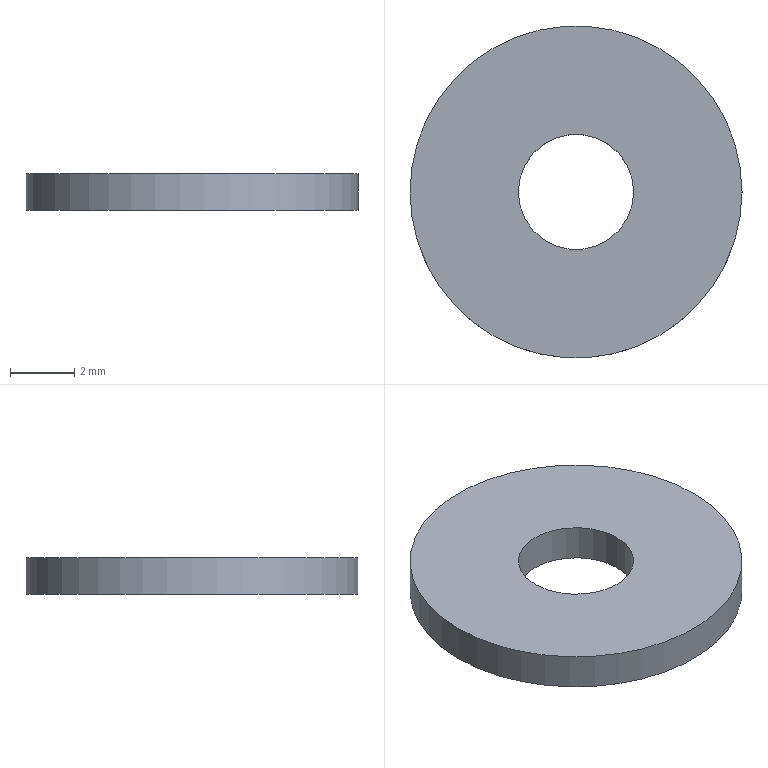Part | NX | features DATUM_CSYS 2, EXTRUDE 1, SKETCH 1 | 1 solid | 4 faces | box 10.312 x 10.312 x 1.143 mm | volume 83.953 mm3 | cylinder 2 | plane 2 | commonest cylinder face diameters 3.581 x1 10.312 x1
STEP:
#1=CARTESIAN_POINT('',(5.156,0.,1.143));
#2=VERTEX_POINT('',#1);
#3=CARTESIAN_POINT('',(0.,0.,1.143));
#4=DIRECTION('',(0.,0.,1.));
#5=DIRECTION('',(1.,0.,0.));
#6=AXIS2_PLACEMENT_3D('',#3,#4,#5);
#7=CIRCLE('',#6,5.156);
#8=EDGE_CURVE('',#2,#2,#7,.T.);
#9=ORIENTED_EDGE('',*,*,#8,.F.);
#10=EDGE_LOOP('',(#9));
#11=FACE_BOUND('',#10,.T.);
#12=CARTESIAN_POINT('',(5.156,0.,0.));
#13=VERTEX_POINT('',#12);
#14=CARTESIAN_POINT('',(0.,0.,0.));
#15=DIRECTION('',(0.,0.,1.));
#16=DIRECTION('',(1.,0.,0.));
#17=AXIS2_PLACEMENT_3D('',#14,#15,#16);
#18=CIRCLE('',#17,5.156);
#19=EDGE_CURVE('',#13,#13,#18,.T.);
#20=ORIENTED_EDGE('',*,*,#19,.T.);
#21=EDGE_LOOP('',(#20));
#22=FACE_BOUND('',#21,.T.);
#23=CARTESIAN_POINT('',(0.,0.,1.143));
#24=DIRECTION('',(0.,0.,-1.));
#25=DIRECTION('',(-1.,0.,0.));
#26=AXIS2_PLACEMENT_3D('',#23,#24,#25);
#27=CYLINDRICAL_SURFACE('',#26,5.156);
#28=ADVANCED_FACE('',(#11,#22),#27,.T.);
#29=CARTESIAN_POINT('',(1.791,0.,1.143));
#30=VERTEX_POINT('',#29);
#31=CARTESIAN_POINT('',(0.,0.,1.143));
#32=DIRECTION('',(0.,0.,1.));
#33=DIRECTION('',(1.,0.,0.));
#34=AXIS2_PLACEMENT_3D('',#31,#32,#33);
#35=CIRCLE('',#34,1.791);
#36=EDGE_CURVE('',#30,#30,#35,.T.);
#37=ORIENTED_EDGE('',*,*,#36,.T.);
#38=EDGE_LOOP('',(#37));
#39=FACE_BOUND('',#38,.T.);
#40=CARTESIAN_POINT('',(1.791,0.,0.));
#41=VERTEX_POINT('',#40);
#42=CARTESIAN_POINT('',(0.,0.,0.));
#43=DIRECTION('',(0.,0.,1.));
#44=DIRECTION('',(1.,0.,0.));
#45=AXIS2_PLACEMENT_3D('',#42,#43,#44);
#46=CIRCLE('',#45,1.791);
#47=EDGE_CURVE('',#41,#41,#46,.T.);
#48=ORIENTED_EDGE('',*,*,#47,.F.);
#49=EDGE_LOOP('',(#48));
#50=FACE_BOUND('',#49,.T.);
#51=CARTESIAN_POINT('',(0.,0.,1.143));
#52=DIRECTION('',(0.,0.,-1.));
#53=DIRECTION('',(-1.,0.,0.));
#54=AXIS2_PLACEMENT_3D('',#51,#52,#53);
#55=CYLINDRICAL_SURFACE('',#54,1.791);
#56=ADVANCED_FACE('',(#39,#50),#55,.F.);
#57=ORIENTED_EDGE('',*,*,#8,.T.);
#58=EDGE_LOOP('',(#57));
#59=FACE_BOUND('',#58,.T.);
#60=ORIENTED_EDGE('',*,*,#36,.F.);
#61=EDGE_LOOP('',(#60));
#62=FACE_BOUND('',#61,.T.);
#63=CARTESIAN_POINT('',(0.,0.,1.143));
#64=DIRECTION('',(0.,0.,1.));
#65=DIRECTION('',(1.,0.,0.));
#66=AXIS2_PLACEMENT_3D('',#63,#64,#65);
#67=PLANE('',#66);
#68=ADVANCED_FACE('',(#59,#62),#67,.T.);
#69=ORIENTED_EDGE('',*,*,#19,.F.);
#70=EDGE_LOOP('',(#69));
#71=FACE_BOUND('',#70,.T.);
#72=ORIENTED_EDGE('',*,*,#47,.T.);
#73=EDGE_LOOP('',(#72));
#74=FACE_BOUND('',#73,.T.);
#75=CARTESIAN_POINT('',(0.,0.,0.));
#76=DIRECTION('',(0.,0.,1.));
#77=DIRECTION('',(1.,0.,0.));
#78=AXIS2_PLACEMENT_3D('',#75,#76,#77);
#79=PLANE('',#78);
#80=ADVANCED_FACE('',(#71,#74),#79,.F.);
#81=CLOSED_SHELL('',(#28,#56,#68,#80));
#82=MANIFOLD_SOLID_BREP('',#81);
#83=(LENGTH_UNIT()NAMED_UNIT(*)SI_UNIT(.MILLI.,.METRE.));
#84=UNCERTAINTY_MEASURE_WITH_UNIT(LENGTH_MEASURE(0.00001),#83,'','');
#85=(NAMED_UNIT(*)PLANE_ANGLE_UNIT()SI_UNIT($,.RADIAN.));
#86=(NAMED_UNIT(*)SI_UNIT($,.STERADIAN.)SOLID_ANGLE_UNIT());
#87=(GEOMETRIC_REPRESENTATION_CONTEXT(3)GLOBAL_UNCERTAINTY_ASSIGNED_CONTEXT((#84))GLOBAL_UNIT_ASSIGNED_CONTEXT((#83,#85,#86))REPRESENTATION_CONTEXT('',''));
#88=ADVANCED_BREP_SHAPE_REPRESENTATION('',(#82),#87);